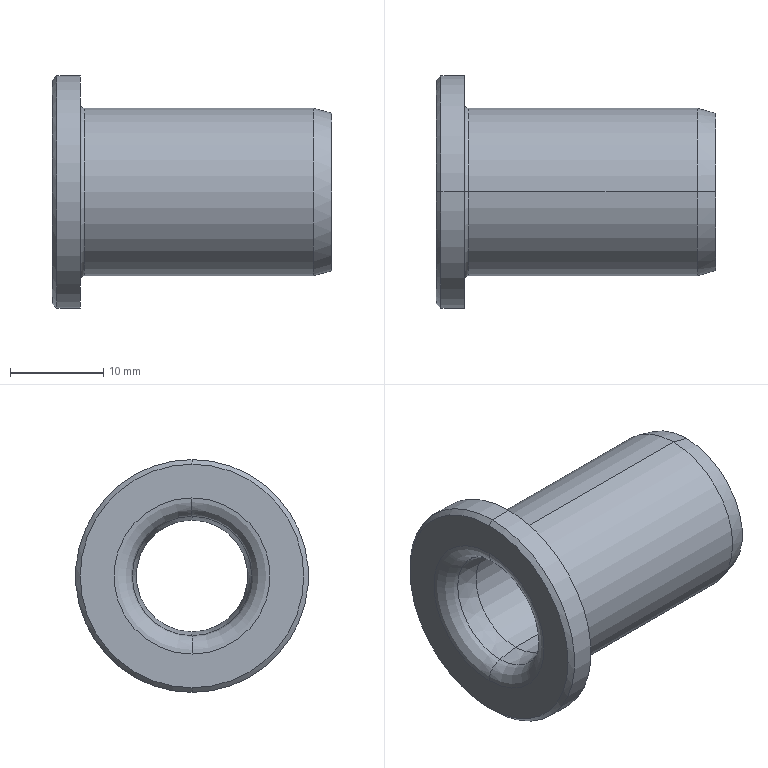Part | STEP file | 001-009-OFN01-d12-L30 | 1 solid | 23 faces | box 30 x 25 x 25 mm | volume 4819 mm3 | cone 8 | torus 6 | cylinder 6 | plane 3 | commonest cylinder face diameters 12 x2 18 x2 25 x2
STEP:
#1=CARTESIAN_POINT('',(0.,0.,0.));
#2=DIRECTION('',(0.,0.,1.));
#3=DIRECTION('',(1.,0.,0.));
#4=AXIS2_PLACEMENT_3D('',#1,#2,#3);
#5=CARTESIAN_POINT('',(0.,0.,-12.));
#6=VERTEX_POINT('',#5);
#7=CARTESIAN_POINT('',(0.,0.,12.));
#8=VERTEX_POINT('',#7);
#9=CARTESIAN_POINT('',(0.,0.,0.));
#10=DIRECTION('',(1.,0.,0.));
#11=DIRECTION('',(0.,0.,-1.));
#12=AXIS2_PLACEMENT_3D('',#9,#10,#11);
#13=CIRCLE('',#12,12.);
#14=CARTESIAN_POINT('',(0.5,0.,0.));
#15=DIRECTION('',(1.,0.,0.));
#16=DIRECTION('',(0.,0.,-1.));
#17=AXIS2_PLACEMENT_3D('',#14,#15,#16);
#18=CONICAL_SURFACE('',#17,12.5,0.7854);
#19=CARTESIAN_POINT('',(0.,-0.5));
#20=DIRECTION('',(1.,0.));
#21=VECTOR('',#20,1.);
#22=LINE('',#19,#21);
#23=(GEOMETRIC_REPRESENTATION_CONTEXT(2)PARAMETRIC_REPRESENTATION_CONTEXT()REPRESENTATION_CONTEXT('',''));
#24=DEFINITIONAL_REPRESENTATION('',(#22),#23);
#25=PCURVE('',#18,#24);
#26=CARTESIAN_POINT('',(0.,12.,0.));
#27=DIRECTION('',(-1.,0.,0.));
#28=DIRECTION('',(0.,0.,1.));
#29=AXIS2_PLACEMENT_3D('',#26,#27,#28);
#30=PLANE('',#29);
#31=CARTESIAN_POINT('',(-12.,-12.));
#32=CARTESIAN_POINT('',(-12.,8.785));
#33=CARTESIAN_POINT('',(6.,-1.608));
#34=CARTESIAN_POINT('',(24.,-12.));
#35=CARTESIAN_POINT('',(6.,-22.392));
#36=CARTESIAN_POINT('',(-12.,-32.785));
#37=CARTESIAN_POINT('',(-12.,-12.));
#38=(BOUNDED_CURVE()B_SPLINE_CURVE(2,(#31,#32,#33,#34,#35,#36,#37),.UNSPECIFIED.,.T.,.F.)B_SPLINE_CURVE_WITH_KNOTS((1,2,2,2,2,1),(-2.094,0.,2.094,4.189,6.283,8.378),.UNSPECIFIED.)CURVE()GEOMETRIC_REPRESENTATION_ITEM()RATIONAL_B_SPLINE_CURVE((1.,0.5,1.,0.5,1.,0.5,1.))REPRESENTATION_ITEM(''));
#39=(GEOMETRIC_REPRESENTATION_CONTEXT(2)PARAMETRIC_REPRESENTATION_CONTEXT()REPRESENTATION_CONTEXT('',''));
#40=DEFINITIONAL_REPRESENTATION('',(#38),#39);
#41=PCURVE('',#30,#40);
#42=SURFACE_CURVE('',#13,(#25,#41),.PCURVE_S1.);
#43=EDGE_CURVE('',#6,#8,#42,.T.);
#44=ORIENTED_EDGE('',*,*,#43,.T.);
#45=CARTESIAN_POINT('',(0.5,0.,12.5));
#46=VERTEX_POINT('',#45);
#47=CARTESIAN_POINT('',(0.5,0.,12.5));
#48=DIRECTION('',(0.7071,0.,0.7071));
#49=VECTOR('',#48,1.);
#50=LINE('',#47,#49);
#51=CARTESIAN_POINT('',(3.142,0.));
#52=DIRECTION('',(0.,1.));
#53=VECTOR('',#52,1.);
#54=LINE('',#51,#53);
#55=(GEOMETRIC_REPRESENTATION_CONTEXT(2)PARAMETRIC_REPRESENTATION_CONTEXT()REPRESENTATION_CONTEXT('',''));
#56=DEFINITIONAL_REPRESENTATION('',(#54),#55);
#57=PCURVE('',#18,#56);
#58=CARTESIAN_POINT('',(0.5,0.,0.));
#59=DIRECTION('',(1.,0.,0.));
#60=DIRECTION('',(0.,0.,-1.));
#61=AXIS2_PLACEMENT_3D('',#58,#59,#60);
#62=CONICAL_SURFACE('',#61,12.5,0.7854);
#63=CARTESIAN_POINT('',(3.142,0.));
#64=DIRECTION('',(0.,1.));
#65=VECTOR('',#64,1.);
#66=LINE('',#63,#65);
#67=(GEOMETRIC_REPRESENTATION_CONTEXT(2)PARAMETRIC_REPRESENTATION_CONTEXT()REPRESENTATION_CONTEXT('',''));
#68=DEFINITIONAL_REPRESENTATION('',(#66),#67);
#69=PCURVE('',#62,#68);
#70=SURFACE_CURVE('',#50,(#57,#69),.PCURVE_S1.);
#71=EDGE_CURVE('',#8,#46,#70,.T.);
#72=ORIENTED_EDGE('',*,*,#71,.T.);
#73=CARTESIAN_POINT('',(0.5,0.,-12.5));
#74=VERTEX_POINT('',#73);
#75=CARTESIAN_POINT('',(0.5,0.,0.));
#76=DIRECTION('',(1.,0.,0.));
#77=DIRECTION('',(0.,0.,-1.));
#78=AXIS2_PLACEMENT_3D('',#75,#76,#77);
#79=CIRCLE('',#78,12.5);
#80=CARTESIAN_POINT('',(0.,0.));
#81=DIRECTION('',(1.,0.));
#82=VECTOR('',#81,1.);
#83=LINE('',#80,#82);
#84=(GEOMETRIC_REPRESENTATION_CONTEXT(2)PARAMETRIC_REPRESENTATION_CONTEXT()REPRESENTATION_CONTEXT('',''));
#85=DEFINITIONAL_REPRESENTATION('',(#83),#84);
#86=PCURVE('',#18,#85);
#87=CARTESIAN_POINT('',(30.,0.,0.));
#88=DIRECTION('',(-1.,0.,0.));
#89=DIRECTION('',(0.,0.,-1.));
#90=AXIS2_PLACEMENT_3D('',#87,#88,#89);
#91=CYLINDRICAL_SURFACE('',#90,12.5);
#92=CARTESIAN_POINT('',(6.283,29.5));
#93=DIRECTION('',(-1.,0.));
#94=VECTOR('',#93,1.);
#95=LINE('',#92,#94);
#96=(GEOMETRIC_REPRESENTATION_CONTEXT(2)PARAMETRIC_REPRESENTATION_CONTEXT()REPRESENTATION_CONTEXT('',''));
#97=DEFINITIONAL_REPRESENTATION('',(#95),#96);
#98=PCURVE('',#91,#97);
#99=SURFACE_CURVE('',#79,(#86,#98),.PCURVE_S1.);
#100=EDGE_CURVE('',#74,#46,#99,.T.);
#101=ORIENTED_EDGE('',*,*,#100,.F.);
#102=CARTESIAN_POINT('',(0.5,0.,-12.5));
#103=DIRECTION('',(0.7071,0.,-0.7071));
#104=VECTOR('',#103,1.);
#105=LINE('',#102,#104);
#106=CARTESIAN_POINT('',(0.,0.));
#107=DIRECTION('',(0.,1.));
#108=VECTOR('',#107,1.);
#109=LINE('',#106,#108);
#110=(GEOMETRIC_REPRESENTATION_CONTEXT(2)PARAMETRIC_REPRESENTATION_CONTEXT()REPRESENTATION_CONTEXT('',''));
#111=DEFINITIONAL_REPRESENTATION('',(#109),#110);
#112=PCURVE('',#18,#111);
#113=CARTESIAN_POINT('',(6.283,0.));
#114=DIRECTION('',(0.,1.));
#115=VECTOR('',#114,1.);
#116=LINE('',#113,#115);
#117=(GEOMETRIC_REPRESENTATION_CONTEXT(2)PARAMETRIC_REPRESENTATION_CONTEXT()REPRESENTATION_CONTEXT('',''));
#118=DEFINITIONAL_REPRESENTATION('',(#116),#117);
#119=PCURVE('',#62,#118);
#120=SURFACE_CURVE('',#105,(#112,#119),.PCURVE_S1.);
#121=EDGE_CURVE('',#6,#74,#120,.T.);
#122=ORIENTED_EDGE('',*,*,#121,.F.);
#123=EDGE_LOOP('',(#44,#72,#101,#122));
#124=FACE_BOUND('',#123,.T.);
#125=ADVANCED_FACE('',(#124),#18,.T.);
#126=CARTESIAN_POINT('',(1.653,0.,-6.414));
#127=VERTEX_POINT('',#126);
#128=CARTESIAN_POINT('',(1.653,0.,6.414));
#129=VERTEX_POINT('',#128);
#130=CARTESIAN_POINT('',(1.653,0.,0.));
#131=DIRECTION('',(1.,0.,0.));
#132=DIRECTION('',(0.,0.,-1.));
#133=AXIS2_PLACEMENT_3D('',#130,#131,#132);
#134=CIRCLE('',#133,6.414);
#135=CARTESIAN_POINT('',(2.,0.,0.));
#136=DIRECTION('',(1.,0.,0.));
#137=DIRECTION('',(0.,0.,-1.));
#138=AXIS2_PLACEMENT_3D('',#135,#136,#137);
#139=TOROIDAL_SURFACE('',#138,8.384,2.);
#140=CARTESIAN_POINT('',(0.,3.316));
#141=DIRECTION('',(1.,0.));
#142=VECTOR('',#141,1.);
#143=LINE('',#140,#142);
#144=(GEOMETRIC_REPRESENTATION_CONTEXT(2)PARAMETRIC_REPRESENTATION_CONTEXT()REPRESENTATION_CONTEXT('',''));
#145=DEFINITIONAL_REPRESENTATION('',(#143),#144);
#146=PCURVE('',#139,#145);
#147=CARTESIAN_POINT('',(1.653,0.,0.));
#148=DIRECTION('',(-1.,0.,0.));
#149=DIRECTION('',(0.,0.,1.));
#150=AXIS2_PLACEMENT_3D('',#147,#148,#149);
#151=CONICAL_SURFACE('',#150,6.414,0.1745);
#152=CARTESIAN_POINT('',(3.142,0.));
#153=DIRECTION('',(-1.,0.));
#154=VECTOR('',#153,1.);
#155=LINE('',#152,#154);
#156=(GEOMETRIC_REPRESENTATION_CONTEXT(2)PARAMETRIC_REPRESENTATION_CONTEXT()REPRESENTATION_CONTEXT('',''));
#157=DEFINITIONAL_REPRESENTATION('',(#155),#156);
#158=PCURVE('',#151,#157);
#159=SURFACE_CURVE('',#134,(#146,#158),.PCURVE_S1.);
#160=EDGE_CURVE('',#127,#129,#159,.T.);
#161=ORIENTED_EDGE('',*,*,#160,.T.);
#162=CARTESIAN_POINT('',(0.,0.,8.384));
#163=VERTEX_POINT('',#162);
#164=CARTESIAN_POINT('',(2.,0.,8.384));
#165=DIRECTION('',(0.,1.,0.));
#166=DIRECTION('',(0.,0.,1.));
#167=AXIS2_PLACEMENT_3D('',#164,#165,#166);
#168=CIRCLE('',#167,2.);
#169=CARTESIAN_POINT('',(3.142,0.));
#170=DIRECTION('',(0.,1.));
#171=VECTOR('',#170,1.);
#172=LINE('',#169,#171);
#173=(GEOMETRIC_REPRESENTATION_CONTEXT(2)PARAMETRIC_REPRESENTATION_CONTEXT()REPRESENTATION_CONTEXT('',''));
#174=DEFINITIONAL_REPRESENTATION('',(#172),#173);
#175=PCURVE('',#139,#174);
#176=CARTESIAN_POINT('',(2.,0.,0.));
#177=DIRECTION('',(1.,0.,0.));
#178=DIRECTION('',(0.,0.,-1.));
#179=AXIS2_PLACEMENT_3D('',#176,#177,#178);
#180=TOROIDAL_SURFACE('',#179,8.384,2.);
#181=CARTESIAN_POINT('',(3.142,0.));
#182=DIRECTION('',(0.,1.));
#183=VECTOR('',#182,1.);
#184=LINE('',#181,#183);
#185=(GEOMETRIC_REPRESENTATION_CONTEXT(2)PARAMETRIC_REPRESENTATION_CONTEXT()REPRESENTATION_CONTEXT('',''));
#186=DEFINITIONAL_REPRESENTATION('',(#184),#185);
#187=PCURVE('',#180,#186);
#188=SURFACE_CURVE('',#168,(#175,#187),.PCURVE_S1.);
#189=EDGE_CURVE('',#129,#163,#188,.T.);
#190=ORIENTED_EDGE('',*,*,#189,.T.);
#191=CARTESIAN_POINT('',(0.,0.,-8.384));
#192=VERTEX_POINT('',#191);
#193=CARTESIAN_POINT('',(0.,0.,0.));
#194=DIRECTION('',(1.,0.,0.));
#195=DIRECTION('',(0.,0.,-1.));
#196=AXIS2_PLACEMENT_3D('',#193,#194,#195);
#197=CIRCLE('',#196,8.384);
#198=CARTESIAN_POINT('',(0.,4.712));
#199=DIRECTION('',(1.,0.));
#200=VECTOR('',#199,1.);
#201=LINE('',#198,#200);
#202=(GEOMETRIC_REPRESENTATION_CONTEXT(2)PARAMETRIC_REPRESENTATION_CONTEXT()REPRESENTATION_CONTEXT('',''));
#203=DEFINITIONAL_REPRESENTATION('',(#201),#202);
#204=PCURVE('',#139,#203);
#205=CARTESIAN_POINT('',(-8.384,-12.));
#206=CARTESIAN_POINT('',(-8.384,2.521));
#207=CARTESIAN_POINT('',(4.192,-4.74));
#208=CARTESIAN_POINT('',(16.767,-12.));
#209=CARTESIAN_POINT('',(4.192,-19.26));
#210=CARTESIAN_POINT('',(-8.384,-26.521));
#211=CARTESIAN_POINT('',(-8.384,-12.));
#212=(BOUNDED_CURVE()B_SPLINE_CURVE(2,(#205,#206,#207,#208,#209,#210,#211),.UNSPECIFIED.,.T.,.F.)B_SPLINE_CURVE_WITH_KNOTS((1,2,2,2,2,1),(-2.094,0.,2.094,4.189,6.283,8.378),.UNSPECIFIED.)CURVE()GEOMETRIC_REPRESENTATION_ITEM()RATIONAL_B_SPLINE_CURVE((1.,0.5,1.,0.5,1.,0.5,1.))REPRESENTATION_ITEM(''));
#213=(GEOMETRIC_REPRESENTATION_CONTEXT(2)PARAMETRIC_REPRESENTATION_CONTEXT()REPRESENTATION_CONTEXT('',''));
#214=DEFINITIONAL_REPRESENTATION('',(#212),#213);
#215=PCURVE('',#30,#214);
#216=SURFACE_CURVE('',#197,(#204,#215),.PCURVE_S1.);
#217=EDGE_CURVE('',#192,#163,#216,.T.);
#218=ORIENTED_EDGE('',*,*,#217,.F.);
#219=CARTESIAN_POINT('',(2.,0.,-8.384));
#220=DIRECTION('',(0.,-1.,0.));
#221=DIRECTION('',(0.,0.,-1.));
#222=AXIS2_PLACEMENT_3D('',#219,#220,#221);
#223=CIRCLE('',#222,2.);
#224=CARTESIAN_POINT('',(0.,0.));
#225=DIRECTION('',(0.,1.));
#226=VECTOR('',#225,1.);
#227=LINE('',#224,#226);
#228=(GEOMETRIC_REPRESENTATION_CONTEXT(2)PARAMETRIC_REPRESENTATION_CONTEXT()REPRESENTATION_CONTEXT('',''));
#229=DEFINITIONAL_REPRESENTATION('',(#227),#228);
#230=PCURVE('',#139,#229);
#231=CARTESIAN_POINT('',(6.283,0.));
#232=DIRECTION('',(0.,1.));
#233=VECTOR('',#232,1.);
#234=LINE('',#231,#233);
#235=(GEOMETRIC_REPRESENTATION_CONTEXT(2)PARAMETRIC_REPRESENTATION_CONTEXT()REPRESENTATION_CONTEXT('',''));
#236=DEFINITIONAL_REPRESENTATION('',(#234),#235);
#237=PCURVE('',#180,#236);
#238=SURFACE_CURVE('',#223,(#230,#237),.PCURVE_S1.);
#239=EDGE_CURVE('',#127,#192,#238,.T.);
#240=ORIENTED_EDGE('',*,*,#239,.F.);
#241=EDGE_LOOP('',(#161,#190,#218,#240));
#242=FACE_BOUND('',#241,.T.);
#243=ADVANCED_FACE('',(#242),#139,.T.);
#244=CARTESIAN_POINT('',(4.,0.,6.));
#245=VERTEX_POINT('',#244);
#246=CARTESIAN_POINT('',(1.653,0.,6.414));
#247=DIRECTION('',(-0.9848,0.,0.1736));
#248=VECTOR('',#247,1.);
#249=LINE('',#246,#248);
#250=CARTESIAN_POINT('',(1.653,0.,0.));
#251=DIRECTION('',(-1.,0.,0.));
#252=DIRECTION('',(0.,0.,1.));
#253=AXIS2_PLACEMENT_3D('',#250,#251,#252);
#254=CONICAL_SURFACE('',#253,6.414,0.1745);
#255=CARTESIAN_POINT('',(6.283,0.));
#256=DIRECTION('',(0.,1.));
#257=VECTOR('',#256,1.);
#258=LINE('',#255,#257);
#259=(GEOMETRIC_REPRESENTATION_CONTEXT(2)PARAMETRIC_REPRESENTATION_CONTEXT()REPRESENTATION_CONTEXT('',''));
#260=DEFINITIONAL_REPRESENTATION('',(#258),#259);
#261=PCURVE('',#254,#260);
#262=CARTESIAN_POINT('',(0.,0.));
#263=DIRECTION('',(0.,1.));
#264=VECTOR('',#263,1.);
#265=LINE('',#262,#264);
#266=(GEOMETRIC_REPRESENTATION_CONTEXT(2)PARAMETRIC_REPRESENTATION_CONTEXT()REPRESENTATION_CONTEXT('',''));
#267=DEFINITIONAL_REPRESENTATION('',(#265),#266);
#268=PCURVE('',#151,#267);
#269=SURFACE_CURVE('',#249,(#261,#268),.PCURVE_S1.);
#270=EDGE_CURVE('',#245,#129,#269,.T.);
#271=ORIENTED_EDGE('',*,*,#270,.T.);
#272=CARTESIAN_POINT('',(1.653,0.,0.));
#273=DIRECTION('',(1.,0.,0.));
#274=DIRECTION('',(0.,0.,-1.));
#275=AXIS2_PLACEMENT_3D('',#272,#273,#274);
#276=CIRCLE('',#275,6.414);
#277=CARTESIAN_POINT('',(9.425,0.));
#278=DIRECTION('',(-1.,0.));
#279=VECTOR('',#278,1.);
#280=LINE('',#277,#279);
#281=(GEOMETRIC_REPRESENTATION_CONTEXT(2)PARAMETRIC_REPRESENTATION_CONTEXT()REPRESENTATION_CONTEXT('',''));
#282=DEFINITIONAL_REPRESENTATION('',(#280),#281);
#283=PCURVE('',#254,#282);
#284=CARTESIAN_POINT('',(0.,3.316));
#285=DIRECTION('',(1.,0.));
#286=VECTOR('',#285,1.);
#287=LINE('',#284,#286);
#288=(GEOMETRIC_REPRESENTATION_CONTEXT(2)PARAMETRIC_REPRESENTATION_CONTEXT()REPRESENTATION_CONTEXT('',''));
#289=DEFINITIONAL_REPRESENTATION('',(#287),#288);
#290=PCURVE('',#180,#289);
#291=SURFACE_CURVE('',#276,(#283,#290),.PCURVE_S1.);
#292=EDGE_CURVE('',#129,#127,#291,.T.);
#293=ORIENTED_EDGE('',*,*,#292,.T.);
#294=CARTESIAN_POINT('',(4.,0.,-6.));
#295=VERTEX_POINT('',#294);
#296=CARTESIAN_POINT('',(1.653,0.,-6.414));
#297=DIRECTION('',(-0.9848,0.,-0.1736));
#298=VECTOR('',#297,1.);
#299=LINE('',#296,#298);
#300=CARTESIAN_POINT('',(3.142,0.));
#301=DIRECTION('',(0.,1.));
#302=VECTOR('',#301,1.);
#303=LINE('',#300,#302);
#304=(GEOMETRIC_REPRESENTATION_CONTEXT(2)PARAMETRIC_REPRESENTATION_CONTEXT()REPRESENTATION_CONTEXT('',''));
#305=DEFINITIONAL_REPRESENTATION('',(#303),#304);
#306=PCURVE('',#254,#305);
#307=CARTESIAN_POINT('',(3.142,0.));
#308=DIRECTION('',(0.,1.));
#309=VECTOR('',#308,1.);
#310=LINE('',#307,#309);
#311=(GEOMETRIC_REPRESENTATION_CONTEXT(2)PARAMETRIC_REPRESENTATION_CONTEXT()REPRESENTATION_CONTEXT('',''));
#312=DEFINITIONAL_REPRESENTATION('',(#310),#311);
#313=PCURVE('',#151,#312);
#314=SURFACE_CURVE('',#299,(#306,#313),.PCURVE_S1.);
#315=EDGE_CURVE('',#295,#127,#314,.T.);
#316=ORIENTED_EDGE('',*,*,#315,.F.);
#317=CARTESIAN_POINT('',(4.,0.,0.));
#318=DIRECTION('',(1.,0.,0.));
#319=DIRECTION('',(0.,0.,-1.));
#320=AXIS2_PLACEMENT_3D('',#317,#318,#319);
#321=CIRCLE('',#320,6.);
#322=CARTESIAN_POINT('',(9.425,-2.347));
#323=DIRECTION('',(-1.,0.));
#324=VECTOR('',#323,1.);
#325=LINE('',#322,#324);
#326=(GEOMETRIC_REPRESENTATION_CONTEXT(2)PARAMETRIC_REPRESENTATION_CONTEXT()REPRESENTATION_CONTEXT('',''));
#327=DEFINITIONAL_REPRESENTATION('',(#325),#326);
#328=PCURVE('',#254,#327);
#329=CARTESIAN_POINT('',(30.,0.,0.));
#330=DIRECTION('',(-1.,0.,0.));
#331=DIRECTION('',(0.,0.,-1.));
#332=AXIS2_PLACEMENT_3D('',#329,#330,#331);
#333=CYLINDRICAL_SURFACE('',#332,6.);
#334=CARTESIAN_POINT('',(6.283,26.));
#335=DIRECTION('',(-1.,0.));
#336=VECTOR('',#335,1.);
#337=LINE('',#334,#336);
#338=(GEOMETRIC_REPRESENTATION_CONTEXT(2)PARAMETRIC_REPRESENTATION_CONTEXT()REPRESENTATION_CONTEXT('',''));
#339=DEFINITIONAL_REPRESENTATION('',(#337),#338);
#340=PCURVE('',#333,#339);
#341=SURFACE_CURVE('',#321,(#328,#340),.PCURVE_S1.);
#342=EDGE_CURVE('',#245,#295,#341,.T.);
#343=ORIENTED_EDGE('',*,*,#342,.F.);
#344=EDGE_LOOP('',(#271,#293,#316,#343));
#345=FACE_BOUND('',#344,.F.);
#346=ADVANCED_FACE('',(#345),#254,.F.);
#347=CARTESIAN_POINT('',(28.,0.,-6.));
#348=VERTEX_POINT('',#347);
#349=CARTESIAN_POINT('',(30.,0.,-6.));
#350=DIRECTION('',(-1.,0.,0.));
#351=VECTOR('',#350,1.);
#352=LINE('',#349,#351);
#353=CARTESIAN_POINT('',(30.,0.,0.));
#354=DIRECTION('',(-1.,0.,0.));
#355=DIRECTION('',(0.,0.,-1.));
#356=AXIS2_PLACEMENT_3D('',#353,#354,#355);
#357=CYLINDRICAL_SURFACE('',#356,6.);
#358=CARTESIAN_POINT('',(6.283,0.));
#359=DIRECTION('',(0.,1.));
#360=VECTOR('',#359,1.);
#361=LINE('',#358,#360);
#362=(GEOMETRIC_REPRESENTATION_CONTEXT(2)PARAMETRIC_REPRESENTATION_CONTEXT()REPRESENTATION_CONTEXT('',''));
#363=DEFINITIONAL_REPRESENTATION('',(#361),#362);
#364=PCURVE('',#357,#363);
#365=CARTESIAN_POINT('',(0.,0.));
#366=DIRECTION('',(0.,1.));
#367=VECTOR('',#366,1.);
#368=LINE('',#365,#367);
#369=(GEOMETRIC_REPRESENTATION_CONTEXT(2)PARAMETRIC_REPRESENTATION_CONTEXT()REPRESENTATION_CONTEXT('',''));
#370=DEFINITIONAL_REPRESENTATION('',(#368),#369);
#371=PCURVE('',#333,#370);
#372=SURFACE_CURVE('',#352,(#364,#371),.PCURVE_S1.);
#373=EDGE_CURVE('',#348,#295,#372,.T.);
#374=ORIENTED_EDGE('',*,*,#373,.T.);
#375=CARTESIAN_POINT('',(4.,0.,0.));
#376=DIRECTION('',(1.,0.,0.));
#377=DIRECTION('',(0.,0.,-1.));
#378=AXIS2_PLACEMENT_3D('',#375,#376,#377);
#379=CIRCLE('',#378,6.);
#380=CARTESIAN_POINT('',(6.283,26.));
#381=DIRECTION('',(-1.,0.));
#382=VECTOR('',#381,1.);
#383=LINE('',#380,#382);
#384=(GEOMETRIC_REPRESENTATION_CONTEXT(2)PARAMETRIC_REPRESENTATION_CONTEXT()REPRESENTATION_CONTEXT('',''));
#385=DEFINITIONAL_REPRESENTATION('',(#383),#384);
#386=PCURVE('',#357,#385);
#387=CARTESIAN_POINT('',(3.142,-2.347));
#388=DIRECTION('',(-1.,0.));
#389=VECTOR('',#388,1.);
#390=LINE('',#387,#389);
#391=(GEOMETRIC_REPRESENTATION_CONTEXT(2)PARAMETRIC_REPRESENTATION_CONTEXT()REPRESENTATION_CONTEXT('',''));
#392=DEFINITIONAL_REPRESENTATION('',(#390),#391);
#393=PCURVE('',#151,#392);
#394=SURFACE_CURVE('',#379,(#386,#393),.PCURVE_S1.);
#395=EDGE_CURVE('',#295,#245,#394,.T.);
#396=ORIENTED_EDGE('',*,*,#395,.T.);
#397=CARTESIAN_POINT('',(28.,0.,6.));
#398=VERTEX_POINT('',#397);
#399=CARTESIAN_POINT('',(30.,0.,6.));
#400=DIRECTION('',(-1.,0.,0.));
#401=VECTOR('',#400,1.);
#402=LINE('',#399,#401);
#403=CARTESIAN_POINT('',(3.142,0.));
#404=DIRECTION('',(0.,1.));
#405=VECTOR('',#404,1.);
#406=LINE('',#403,#405);
#407=(GEOMETRIC_REPRESENTATION_CONTEXT(2)PARAMETRIC_REPRESENTATION_CONTEXT()REPRESENTATION_CONTEXT('',''));
#408=DEFINITIONAL_REPRESENTATION('',(#406),#407);
#409=PCURVE('',#357,#408);
#410=CARTESIAN_POINT('',(3.142,0.));
#411=DIRECTION('',(0.,1.));
#412=VECTOR('',#411,1.);
#413=LINE('',#410,#412);
#414=(GEOMETRIC_REPRESENTATION_CONTEXT(2)PARAMETRIC_REPRESENTATION_CONTEXT()REPRESENTATION_CONTEXT('',''));
#415=DEFINITIONAL_REPRESENTATION('',(#413),#414);
#416=PCURVE('',#333,#415);
#417=SURFACE_CURVE('',#402,(#409,#416),.PCURVE_S1.);
#418=EDGE_CURVE('',#398,#245,#417,.T.);
#419=ORIENTED_EDGE('',*,*,#418,.F.);
#420=CARTESIAN_POINT('',(28.,0.,0.));
#421=DIRECTION('',(1.,0.,0.));
#422=DIRECTION('',(0.,0.,-1.));
#423=AXIS2_PLACEMENT_3D('',#420,#421,#422);
#424=CIRCLE('',#423,6.);
#425=CARTESIAN_POINT('',(6.283,2.));
#426=DIRECTION('',(-1.,0.));
#427=VECTOR('',#426,1.);
#428=LINE('',#425,#427);
#429=(GEOMETRIC_REPRESENTATION_CONTEXT(2)PARAMETRIC_REPRESENTATION_CONTEXT()REPRESENTATION_CONTEXT('',''));
#430=DEFINITIONAL_REPRESENTATION('',(#428),#429);
#431=PCURVE('',#357,#430);
#432=CARTESIAN_POINT('',(28.,0.,0.));
#433=DIRECTION('',(1.,0.,0.));
#434=DIRECTION('',(0.,0.,-1.));
#435=AXIS2_PLACEMENT_3D('',#432,#433,#434);
#436=CONICAL_SURFACE('',#435,6.,0.1745);
#437=CARTESIAN_POINT('',(0.,0.));
#438=DIRECTION('',(1.,0.));
#439=VECTOR('',#438,1.);
#440=LINE('',#437,#439);
#441=(GEOMETRIC_REPRESENTATION_CONTEXT(2)PARAMETRIC_REPRESENTATION_CONTEXT()REPRESENTATION_CONTEXT('',''));
#442=DEFINITIONAL_REPRESENTATION('',(#440),#441);
#443=PCURVE('',#436,#442);
#444=SURFACE_CURVE('',#424,(#431,#443),.PCURVE_S1.);
#445=EDGE_CURVE('',#348,#398,#444,.T.);
#446=ORIENTED_EDGE('',*,*,#445,.F.);
#447=EDGE_LOOP('',(#374,#396,#419,#446));
#448=FACE_BOUND('',#447,.F.);
#449=ADVANCED_FACE('',(#448),#357,.F.);
#450=CARTESIAN_POINT('',(29.587,0.,-6.28));
#451=VERTEX_POINT('',#450);
#452=CARTESIAN_POINT('',(28.,0.,-6.));
#453=DIRECTION('',(0.9848,0.,-0.1736));
#454=VECTOR('',#453,1.);
#455=LINE('',#452,#454);
#456=CARTESIAN_POINT('',(28.,0.,0.));
#457=DIRECTION('',(1.,0.,0.));
#458=DIRECTION('',(0.,0.,-1.));
#459=AXIS2_PLACEMENT_3D('',#456,#457,#458);
#460=CONICAL_SURFACE('',#459,6.,0.1745);
#461=CARTESIAN_POINT('',(6.283,0.));
#462=DIRECTION('',(0.,1.));
#463=VECTOR('',#462,1.);
#464=LINE('',#461,#463);
#465=(GEOMETRIC_REPRESENTATION_CONTEXT(2)PARAMETRIC_REPRESENTATION_CONTEXT()REPRESENTATION_CONTEXT('',''));
#466=DEFINITIONAL_REPRESENTATION('',(#464),#465);
#467=PCURVE('',#460,#466);
#468=CARTESIAN_POINT('',(0.,0.));
#469=DIRECTION('',(0.,1.));
#470=VECTOR('',#469,1.);
#471=LINE('',#468,#470);
#472=(GEOMETRIC_REPRESENTATION_CONTEXT(2)PARAMETRIC_REPRESENTATION_CONTEXT()REPRESENTATION_CONTEXT('',''));
#473=DEFINITIONAL_REPRESENTATION('',(#471),#472);
#474=PCURVE('',#436,#473);
#475=SURFACE_CURVE('',#455,(#467,#474),.PCURVE_S1.);
#476=EDGE_CURVE('',#348,#451,#475,.T.);
#477=ORIENTED_EDGE('',*,*,#476,.T.);
#478=CARTESIAN_POINT('',(29.587,0.,6.28));
#479=VERTEX_POINT('',#478);
#480=CARTESIAN_POINT('',(29.587,0.,0.));
#481=DIRECTION('',(1.,0.,0.));
#482=DIRECTION('',(0.,0.,-1.));
#483=AXIS2_PLACEMENT_3D('',#480,#481,#482);
#484=CIRCLE('',#483,6.28);
#485=CARTESIAN_POINT('',(0.,1.587));
#486=DIRECTION('',(1.,0.));
#487=VECTOR('',#486,1.);
#488=LINE('',#485,#487);
#489=(GEOMETRIC_REPRESENTATION_CONTEXT(2)PARAMETRIC_REPRESENTATION_CONTEXT()REPRESENTATION_CONTEXT('',''));
#490=DEFINITIONAL_REPRESENTATION('',(#488),#489);
#491=PCURVE('',#460,#490);
#492=CARTESIAN_POINT('',(29.5,0.,0.));
#493=DIRECTION('',(1.,0.,0.));
#494=DIRECTION('',(0.,0.,-1.));
#495=AXIS2_PLACEMENT_3D('',#492,#493,#494);
#496=TOROIDAL_SURFACE('',#495,6.772,0.5);
#497=CARTESIAN_POINT('',(0.,2.967));
#498=DIRECTION('',(1.,0.));
#499=VECTOR('',#498,1.);
#500=LINE('',#497,#499);
#501=(GEOMETRIC_REPRESENTATION_CONTEXT(2)PARAMETRIC_REPRESENTATION_CONTEXT()REPRESENTATION_CONTEXT('',''));
#502=DEFINITIONAL_REPRESENTATION('',(#500),#501);
#503=PCURVE('',#496,#502);
#504=SURFACE_CURVE('',#484,(#491,#503),.PCURVE_S1.);
#505=EDGE_CURVE('',#479,#451,#504,.T.);
#506=ORIENTED_EDGE('',*,*,#505,.F.);
#507=CARTESIAN_POINT('',(28.,0.,6.));
#508=DIRECTION('',(0.9848,0.,0.1736));
#509=VECTOR('',#508,1.);
#510=LINE('',#507,#509);
#511=CARTESIAN_POINT('',(3.142,0.));
#512=DIRECTION('',(0.,1.));
#513=VECTOR('',#512,1.);
#514=LINE('',#511,#513);
#515=(GEOMETRIC_REPRESENTATION_CONTEXT(2)PARAMETRIC_REPRESENTATION_CONTEXT()REPRESENTATION_CONTEXT('',''));
#516=DEFINITIONAL_REPRESENTATION('',(#514),#515);
#517=PCURVE('',#460,#516);
#518=CARTESIAN_POINT('',(3.142,0.));
#519=DIRECTION('',(0.,1.));
#520=VECTOR('',#519,1.);
#521=LINE('',#518,#520);
#522=(GEOMETRIC_REPRESENTATION_CONTEXT(2)PARAMETRIC_REPRESENTATION_CONTEXT()REPRESENTATION_CONTEXT('',''));
#523=DEFINITIONAL_REPRESENTATION('',(#521),#522);
#524=PCURVE('',#436,#523);
#525=SURFACE_CURVE('',#510,(#517,#524),.PCURVE_S1.);
#526=EDGE_CURVE('',#398,#479,#525,.T.);
#527=ORIENTED_EDGE('',*,*,#526,.F.);
#528=CARTESIAN_POINT('',(28.,0.,0.));
#529=DIRECTION('',(1.,0.,0.));
#530=DIRECTION('',(0.,0.,-1.));
#531=AXIS2_PLACEMENT_3D('',#528,#529,#530);
#532=CIRCLE('',#531,6.);
#533=CARTESIAN_POINT('',(0.,0.));
#534=DIRECTION('',(1.,0.));
#535=VECTOR('',#534,1.);
#536=LINE('',#533,#535);
#537=(GEOMETRIC_REPRESENTATION_CONTEXT(2)PARAMETRIC_REPRESENTATION_CONTEXT()REPRESENTATION_CONTEXT('',''));
#538=DEFINITIONAL_REPRESENTATION('',(#536),#537);
#539=PCURVE('',#460,#538);
#540=CARTESIAN_POINT('',(6.283,2.));
#541=DIRECTION('',(-1.,0.));
#542=VECTOR('',#541,1.);
#543=LINE('',#540,#542);
#544=(GEOMETRIC_REPRESENTATION_CONTEXT(2)PARAMETRIC_REPRESENTATION_CONTEXT()REPRESENTATION_CONTEXT('',''));
#545=DEFINITIONAL_REPRESENTATION('',(#543),#544);
#546=PCURVE('',#333,#545);
#547=SURFACE_CURVE('',#532,(#539,#546),.PCURVE_S1.);
#548=EDGE_CURVE('',#398,#348,#547,.T.);
#549=ORIENTED_EDGE('',*,*,#548,.T.);
#550=EDGE_LOOP('',(#477,#506,#527,#549));
#551=FACE_BOUND('',#550,.F.);
#552=ADVANCED_FACE('',(#551),#460,.F.);
#553=CARTESIAN_POINT('',(30.,0.,-6.772));
#554=VERTEX_POINT('',#553);
#555=CARTESIAN_POINT('',(30.,0.,6.772));
#556=VERTEX_POINT('',#555);
#557=CARTESIAN_POINT('',(30.,0.,0.));
#558=DIRECTION('',(1.,0.,0.));
#559=DIRECTION('',(0.,0.,-1.));
#560=AXIS2_PLACEMENT_3D('',#557,#558,#559);
#561=CIRCLE('',#560,6.772);
#562=CARTESIAN_POINT('',(29.5,0.,0.));
#563=DIRECTION('',(1.,0.,0.));
#564=DIRECTION('',(0.,0.,-1.));
#565=AXIS2_PLACEMENT_3D('',#562,#563,#564);
#566=TOROIDAL_SURFACE('',#565,6.772,0.5);
#567=CARTESIAN_POINT('',(0.,1.571));
#568=DIRECTION('',(1.,0.));
#569=VECTOR('',#568,1.);
#570=LINE('',#567,#569);
#571=(GEOMETRIC_REPRESENTATION_CONTEXT(2)PARAMETRIC_REPRESENTATION_CONTEXT()REPRESENTATION_CONTEXT('',''));
#572=DEFINITIONAL_REPRESENTATION('',(#570),#571);
#573=PCURVE('',#566,#572);
#574=CARTESIAN_POINT('',(30.,6.772,0.));
#575=DIRECTION('',(1.,0.,0.));
#576=DIRECTION('',(0.,1.,0.));
#577=AXIS2_PLACEMENT_3D('',#574,#575,#576);
#578=PLANE('',#577);
#579=CARTESIAN_POINT('',(-6.772,0.));
#580=DIRECTION('',(0.,-1.));
#581=AXIS2_PLACEMENT_2D('',#579,#580);
#582=CIRCLE('',#581,6.772);
#583=(GEOMETRIC_REPRESENTATION_CONTEXT(2)PARAMETRIC_REPRESENTATION_CONTEXT()REPRESENTATION_CONTEXT('',''));
#584=DEFINITIONAL_REPRESENTATION('',(#582),#583);
#585=PCURVE('',#578,#584);
#586=SURFACE_CURVE('',#561,(#573,#585),.PCURVE_S1.);
#587=EDGE_CURVE('',#554,#556,#586,.T.);
#588=ORIENTED_EDGE('',*,*,#587,.T.);
#589=CARTESIAN_POINT('',(29.5,0.,6.772));
#590=DIRECTION('',(0.,1.,0.));
#591=DIRECTION('',(0.,0.,1.));
#592=AXIS2_PLACEMENT_3D('',#589,#590,#591);
#593=CIRCLE('',#592,0.5);
#594=CARTESIAN_POINT('',(3.142,0.));
#595=DIRECTION('',(0.,1.));
#596=VECTOR('',#595,1.);
#597=LINE('',#594,#596);
#598=(GEOMETRIC_REPRESENTATION_CONTEXT(2)PARAMETRIC_REPRESENTATION_CONTEXT()REPRESENTATION_CONTEXT('',''));
#599=DEFINITIONAL_REPRESENTATION('',(#597),#598);
#600=PCURVE('',#566,#599);
#601=CARTESIAN_POINT('',(3.142,0.));
#602=DIRECTION('',(0.,1.));
#603=VECTOR('',#602,1.);
#604=LINE('',#601,#603);
#605=(GEOMETRIC_REPRESENTATION_CONTEXT(2)PARAMETRIC_REPRESENTATION_CONTEXT()REPRESENTATION_CONTEXT('',''));
#606=DEFINITIONAL_REPRESENTATION('',(#604),#605);
#607=PCURVE('',#496,#606);
#608=SURFACE_CURVE('',#593,(#600,#607),.PCURVE_S1.);
#609=EDGE_CURVE('',#556,#479,#608,.T.);
#610=ORIENTED_EDGE('',*,*,#609,.T.);
#611=CARTESIAN_POINT('',(29.587,0.,0.));
#612=DIRECTION('',(1.,0.,0.));
#613=DIRECTION('',(0.,0.,-1.));
#614=AXIS2_PLACEMENT_3D('',#611,#612,#613);
#615=CIRCLE('',#614,6.28);
#616=CARTESIAN_POINT('',(0.,2.967));
#617=DIRECTION('',(1.,0.));
#618=VECTOR('',#617,1.);
#619=LINE('',#616,#618);
#620=(GEOMETRIC_REPRESENTATION_CONTEXT(2)PARAMETRIC_REPRESENTATION_CONTEXT()REPRESENTATION_CONTEXT('',''));
#621=DEFINITIONAL_REPRESENTATION('',(#619),#620);
#622=PCURVE('',#566,#621);
#623=CARTESIAN_POINT('',(0.,1.587));
#624=DIRECTION('',(1.,0.));
#625=VECTOR('',#624,1.);
#626=LINE('',#623,#625);
#627=(GEOMETRIC_REPRESENTATION_CONTEXT(2)PARAMETRIC_REPRESENTATION_CONTEXT()REPRESENTATION_CONTEXT('',''));
#628=DEFINITIONAL_REPRESENTATION('',(#626),#627);
#629=PCURVE('',#436,#628);
#630=SURFACE_CURVE('',#615,(#622,#629),.PCURVE_S1.);
#631=EDGE_CURVE('',#451,#479,#630,.T.);
#632=ORIENTED_EDGE('',*,*,#631,.F.);
#633=CARTESIAN_POINT('',(29.5,0.,-6.772));
#634=DIRECTION('',(0.,-1.,0.));
#635=DIRECTION('',(0.,0.,-1.));
#636=AXIS2_PLACEMENT_3D('',#633,#634,#635);
#637=CIRCLE('',#636,0.5);
#638=CARTESIAN_POINT('',(0.,0.));
#639=DIRECTION('',(0.,1.));
#640=VECTOR('',#639,1.);
#641=LINE('',#638,#640);
#642=(GEOMETRIC_REPRESENTATION_CONTEXT(2)PARAMETRIC_REPRESENTATION_CONTEXT()REPRESENTATION_CONTEXT('',''));
#643=DEFINITIONAL_REPRESENTATION('',(#641),#642);
#644=PCURVE('',#566,#643);
#645=CARTESIAN_POINT('',(6.283,0.));
#646=DIRECTION('',(0.,1.));
#647=VECTOR('',#646,1.);
#648=LINE('',#645,#647);
#649=(GEOMETRIC_REPRESENTATION_CONTEXT(2)PARAMETRIC_REPRESENTATION_CONTEXT()REPRESENTATION_CONTEXT('',''));
#650=DEFINITIONAL_REPRESENTATION('',(#648),#649);
#651=PCURVE('',#496,#650);
#652=SURFACE_CURVE('',#637,(#644,#651),.PCURVE_S1.);
#653=EDGE_CURVE('',#554,#451,#652,.T.);
#654=ORIENTED_EDGE('',*,*,#653,.F.);
#655=EDGE_LOOP('',(#588,#610,#632,#654));
#656=FACE_BOUND('',#655,.T.);
#657=ADVANCED_FACE('',(#656),#566,.T.);
#658=CARTESIAN_POINT('',(30.,0.,-8.464));
#659=VERTEX_POINT('',#658);
#660=CARTESIAN_POINT('',(30.,0.,8.464));
#661=VERTEX_POINT('',#660);
#662=CARTESIAN_POINT('',(30.,0.,0.));
#663=DIRECTION('',(1.,0.,0.));
#664=DIRECTION('',(0.,0.,-1.));
#665=AXIS2_PLACEMENT_3D('',#662,#663,#664);
#666=CIRCLE('',#665,8.464);
#667=CARTESIAN_POINT('',(30.,0.,0.));
#668=DIRECTION('',(-1.,0.,0.));
#669=DIRECTION('',(0.,0.,1.));
#670=AXIS2_PLACEMENT_3D('',#667,#668,#669);
#671=CONICAL_SURFACE('',#670,8.464,0.2618);
#672=CARTESIAN_POINT('',(3.142,0.));
#673=DIRECTION('',(-1.,0.));
#674=VECTOR('',#673,1.);
#675=LINE('',#672,#674);
#676=(GEOMETRIC_REPRESENTATION_CONTEXT(2)PARAMETRIC_REPRESENTATION_CONTEXT()REPRESENTATION_CONTEXT('',''));
#677=DEFINITIONAL_REPRESENTATION('',(#675),#676);
#678=PCURVE('',#671,#677);
#679=CARTESIAN_POINT('',(-6.772,0.));
#680=DIRECTION('',(0.,-1.));
#681=AXIS2_PLACEMENT_2D('',#679,#680);
#682=CIRCLE('',#681,8.464);
#683=(GEOMETRIC_REPRESENTATION_CONTEXT(2)PARAMETRIC_REPRESENTATION_CONTEXT()REPRESENTATION_CONTEXT('',''));
#684=DEFINITIONAL_REPRESENTATION('',(#682),#683);
#685=PCURVE('',#578,#684);
#686=SURFACE_CURVE('',#666,(#678,#685),.PCURVE_S1.);
#687=EDGE_CURVE('',#659,#661,#686,.T.);
#688=ORIENTED_EDGE('',*,*,#687,.F.);
#689=CARTESIAN_POINT('',(28.,0.,-9.));
#690=VERTEX_POINT('',#689);
#691=CARTESIAN_POINT('',(30.,0.,-8.464));
#692=DIRECTION('',(-0.9659,0.,-0.2588));
#693=VECTOR('',#692,1.);
#694=LINE('',#691,#693);
#695=CARTESIAN_POINT('',(3.142,0.));
#696=DIRECTION('',(0.,1.));
#697=VECTOR('',#696,1.);
#698=LINE('',#695,#697);
#699=(GEOMETRIC_REPRESENTATION_CONTEXT(2)PARAMETRIC_REPRESENTATION_CONTEXT()REPRESENTATION_CONTEXT('',''));
#700=DEFINITIONAL_REPRESENTATION('',(#698),#699);
#701=PCURVE('',#671,#700);
#702=CARTESIAN_POINT('',(30.,0.,0.));
#703=DIRECTION('',(-1.,0.,0.));
#704=DIRECTION('',(0.,0.,1.));
#705=AXIS2_PLACEMENT_3D('',#702,#703,#704);
#706=CONICAL_SURFACE('',#705,8.464,0.2618);
#707=CARTESIAN_POINT('',(3.142,0.));
#708=DIRECTION('',(0.,1.));
#709=VECTOR('',#708,1.);
#710=LINE('',#707,#709);
#711=(GEOMETRIC_REPRESENTATION_CONTEXT(2)PARAMETRIC_REPRESENTATION_CONTEXT()REPRESENTATION_CONTEXT('',''));
#712=DEFINITIONAL_REPRESENTATION('',(#710),#711);
#713=PCURVE('',#706,#712);
#714=SURFACE_CURVE('',#694,(#701,#713),.PCURVE_S1.);
#715=EDGE_CURVE('',#659,#690,#714,.T.);
#716=ORIENTED_EDGE('',*,*,#715,.T.);
#717=CARTESIAN_POINT('',(28.,0.,9.));
#718=VERTEX_POINT('',#717);
#719=CARTESIAN_POINT('',(28.,0.,0.));
#720=DIRECTION('',(1.,0.,0.));
#721=DIRECTION('',(0.,0.,-1.));
#722=AXIS2_PLACEMENT_3D('',#719,#720,#721);
#723=CIRCLE('',#722,9.);
#724=CARTESIAN_POINT('',(3.142,2.));
#725=DIRECTION('',(-1.,0.));
#726=VECTOR('',#725,1.);
#727=LINE('',#724,#726);
#728=(GEOMETRIC_REPRESENTATION_CONTEXT(2)PARAMETRIC_REPRESENTATION_CONTEXT()REPRESENTATION_CONTEXT('',''));
#729=DEFINITIONAL_REPRESENTATION('',(#727),#728);
#730=PCURVE('',#671,#729);
#731=CARTESIAN_POINT('',(30.,0.,0.));
#732=DIRECTION('',(-1.,0.,0.));
#733=DIRECTION('',(0.,0.,-1.));
#734=AXIS2_PLACEMENT_3D('',#731,#732,#733);
#735=CYLINDRICAL_SURFACE('',#734,9.);
#736=CARTESIAN_POINT('',(6.283,2.));
#737=DIRECTION('',(-1.,0.));
#738=VECTOR('',#737,1.);
#739=LINE('',#736,#738);
#740=(GEOMETRIC_REPRESENTATION_CONTEXT(2)PARAMETRIC_REPRESENTATION_CONTEXT()REPRESENTATION_CONTEXT('',''));
#741=DEFINITIONAL_REPRESENTATION('',(#739),#740);
#742=PCURVE('',#735,#741);
#743=SURFACE_CURVE('',#723,(#730,#742),.PCURVE_S1.);
#744=EDGE_CURVE('',#690,#718,#743,.T.);
#745=ORIENTED_EDGE('',*,*,#744,.T.);
#746=CARTESIAN_POINT('',(30.,0.,8.464));
#747=DIRECTION('',(-0.9659,0.,0.2588));
#748=VECTOR('',#747,1.);
#749=LINE('',#746,#748);
#750=CARTESIAN_POINT('',(0.,0.));
#751=DIRECTION('',(0.,1.));
#752=VECTOR('',#751,1.);
#753=LINE('',#750,#752);
#754=(GEOMETRIC_REPRESENTATION_CONTEXT(2)PARAMETRIC_REPRESENTATION_CONTEXT()REPRESENTATION_CONTEXT('',''));
#755=DEFINITIONAL_REPRESENTATION('',(#753),#754);
#756=PCURVE('',#671,#755);
#757=CARTESIAN_POINT('',(6.283,0.));
#758=DIRECTION('',(0.,1.));
#759=VECTOR('',#758,1.);
#760=LINE('',#757,#759);
#761=(GEOMETRIC_REPRESENTATION_CONTEXT(2)PARAMETRIC_REPRESENTATION_CONTEXT()REPRESENTATION_CONTEXT('',''));
#762=DEFINITIONAL_REPRESENTATION('',(#760),#761);
#763=PCURVE('',#706,#762);
#764=SURFACE_CURVE('',#749,(#756,#763),.PCURVE_S1.);
#765=EDGE_CURVE('',#661,#718,#764,.T.);
#766=ORIENTED_EDGE('',*,*,#765,.F.);
#767=EDGE_LOOP('',(#688,#716,#745,#766));
#768=FACE_BOUND('',#767,.T.);
#769=ADVANCED_FACE('',(#768),#671,.T.);
#770=CARTESIAN_POINT('',(28.,0.,0.));
#771=DIRECTION('',(1.,0.,0.));
#772=DIRECTION('',(0.,0.,-1.));
#773=AXIS2_PLACEMENT_3D('',#770,#771,#772);
#774=CIRCLE('',#773,9.);
#775=CARTESIAN_POINT('',(30.,0.,0.));
#776=DIRECTION('',(-1.,0.,0.));
#777=DIRECTION('',(0.,0.,-1.));
#778=AXIS2_PLACEMENT_3D('',#775,#776,#777);
#779=CYLINDRICAL_SURFACE('',#778,9.);
#780=CARTESIAN_POINT('',(6.283,2.));
#781=DIRECTION('',(-1.,0.));
#782=VECTOR('',#781,1.);
#783=LINE('',#780,#782);
#784=(GEOMETRIC_REPRESENTATION_CONTEXT(2)PARAMETRIC_REPRESENTATION_CONTEXT()REPRESENTATION_CONTEXT('',''));
#785=DEFINITIONAL_REPRESENTATION('',(#783),#784);
#786=PCURVE('',#779,#785);
#787=CARTESIAN_POINT('',(9.425,2.));
#788=DIRECTION('',(-1.,0.));
#789=VECTOR('',#788,1.);
#790=LINE('',#787,#789);
#791=(GEOMETRIC_REPRESENTATION_CONTEXT(2)PARAMETRIC_REPRESENTATION_CONTEXT()REPRESENTATION_CONTEXT('',''));
#792=DEFINITIONAL_REPRESENTATION('',(#790),#791);
#793=PCURVE('',#706,#792);
#794=SURFACE_CURVE('',#774,(#786,#793),.PCURVE_S1.);
#795=EDGE_CURVE('',#718,#690,#794,.T.);
#796=ORIENTED_EDGE('',*,*,#795,.F.);
#797=CARTESIAN_POINT('',(3.5,0.,9.));
#798=VERTEX_POINT('',#797);
#799=CARTESIAN_POINT('',(30.,0.,9.));
#800=DIRECTION('',(-1.,0.,0.));
#801=VECTOR('',#800,1.);
#802=LINE('',#799,#801);
#803=CARTESIAN_POINT('',(3.142,0.));
#804=DIRECTION('',(0.,1.));
#805=VECTOR('',#804,1.);
#806=LINE('',#803,#805);
#807=(GEOMETRIC_REPRESENTATION_CONTEXT(2)PARAMETRIC_REPRESENTATION_CONTEXT()REPRESENTATION_CONTEXT('',''));
#808=DEFINITIONAL_REPRESENTATION('',(#806),#807);
#809=PCURVE('',#779,#808);
#810=CARTESIAN_POINT('',(3.142,0.));
#811=DIRECTION('',(0.,1.));
#812=VECTOR('',#811,1.);
#813=LINE('',#810,#812);
#814=(GEOMETRIC_REPRESENTATION_CONTEXT(2)PARAMETRIC_REPRESENTATION_CONTEXT()REPRESENTATION_CONTEXT('',''));
#815=DEFINITIONAL_REPRESENTATION('',(#813),#814);
#816=PCURVE('',#735,#815);
#817=SURFACE_CURVE('',#802,(#809,#816),.PCURVE_S1.);
#818=EDGE_CURVE('',#718,#798,#817,.T.);
#819=ORIENTED_EDGE('',*,*,#818,.T.);
#820=CARTESIAN_POINT('',(3.5,0.,-9.));
#821=VERTEX_POINT('',#820);
#822=CARTESIAN_POINT('',(3.5,0.,0.));
#823=DIRECTION('',(1.,0.,0.));
#824=DIRECTION('',(0.,0.,-1.));
#825=AXIS2_PLACEMENT_3D('',#822,#823,#824);
#826=CIRCLE('',#825,9.);
#827=CARTESIAN_POINT('',(6.283,26.5));
#828=DIRECTION('',(-1.,0.));
#829=VECTOR('',#828,1.);
#830=LINE('',#827,#829);
#831=(GEOMETRIC_REPRESENTATION_CONTEXT(2)PARAMETRIC_REPRESENTATION_CONTEXT()REPRESENTATION_CONTEXT('',''));
#832=DEFINITIONAL_REPRESENTATION('',(#830),#831);
#833=PCURVE('',#779,#832);
#834=CARTESIAN_POINT('',(3.5,0.,0.));
#835=DIRECTION('',(1.,0.,0.));
#836=DIRECTION('',(0.,0.,-1.));
#837=AXIS2_PLACEMENT_3D('',#834,#835,#836);
#838=TOROIDAL_SURFACE('',#837,9.5,0.5);
#839=CARTESIAN_POINT('',(0.,3.142));
#840=DIRECTION('',(1.,0.));
#841=VECTOR('',#840,1.);
#842=LINE('',#839,#841);
#843=(GEOMETRIC_REPRESENTATION_CONTEXT(2)PARAMETRIC_REPRESENTATION_CONTEXT()REPRESENTATION_CONTEXT('',''));
#844=DEFINITIONAL_REPRESENTATION('',(#842),#843);
#845=PCURVE('',#838,#844);
#846=SURFACE_CURVE('',#826,(#833,#845),.PCURVE_S1.);
#847=EDGE_CURVE('',#798,#821,#846,.T.);
#848=ORIENTED_EDGE('',*,*,#847,.T.);
#849=CARTESIAN_POINT('',(30.,0.,-9.));
#850=DIRECTION('',(-1.,0.,0.));
#851=VECTOR('',#850,1.);
#852=LINE('',#849,#851);
#853=CARTESIAN_POINT('',(0.,0.));
#854=DIRECTION('',(0.,1.));
#855=VECTOR('',#854,1.);
#856=LINE('',#853,#855);
#857=(GEOMETRIC_REPRESENTATION_CONTEXT(2)PARAMETRIC_REPRESENTATION_CONTEXT()REPRESENTATION_CONTEXT('',''));
#858=DEFINITIONAL_REPRESENTATION('',(#856),#857);
#859=PCURVE('',#779,#858);
#860=CARTESIAN_POINT('',(6.283,0.));
#861=DIRECTION('',(0.,1.));
#862=VECTOR('',#861,1.);
#863=LINE('',#860,#862);
#864=(GEOMETRIC_REPRESENTATION_CONTEXT(2)PARAMETRIC_REPRESENTATION_CONTEXT()REPRESENTATION_CONTEXT('',''));
#865=DEFINITIONAL_REPRESENTATION('',(#863),#864);
#866=PCURVE('',#735,#865);
#867=SURFACE_CURVE('',#852,(#859,#866),.PCURVE_S1.);
#868=EDGE_CURVE('',#690,#821,#867,.T.);
#869=ORIENTED_EDGE('',*,*,#868,.F.);
#870=EDGE_LOOP('',(#796,#819,#848,#869));
#871=FACE_BOUND('',#870,.T.);
#872=ADVANCED_FACE('',(#871),#779,.T.);
#873=CARTESIAN_POINT('',(3.,0.,-9.5));
#874=VERTEX_POINT('',#873);
#875=CARTESIAN_POINT('',(3.5,0.,-9.5));
#876=DIRECTION('',(0.,-1.,0.));
#877=DIRECTION('',(0.,0.,-1.));
#878=AXIS2_PLACEMENT_3D('',#875,#876,#877);
#879=CIRCLE('',#878,0.5);
#880=CARTESIAN_POINT('',(6.283,0.));
#881=DIRECTION('',(0.,1.));
#882=VECTOR('',#881,1.);
#883=LINE('',#880,#882);
#884=(GEOMETRIC_REPRESENTATION_CONTEXT(2)PARAMETRIC_REPRESENTATION_CONTEXT()REPRESENTATION_CONTEXT('',''));
#885=DEFINITIONAL_REPRESENTATION('',(#883),#884);
#886=PCURVE('',#838,#885);
#887=CARTESIAN_POINT('',(3.5,0.,0.));
#888=DIRECTION('',(1.,0.,0.));
#889=DIRECTION('',(0.,0.,-1.));
#890=AXIS2_PLACEMENT_3D('',#887,#888,#889);
#891=TOROIDAL_SURFACE('',#890,9.5,0.5);
#892=CARTESIAN_POINT('',(0.,0.));
#893=DIRECTION('',(0.,1.));
#894=VECTOR('',#893,1.);
#895=LINE('',#892,#894);
#896=(GEOMETRIC_REPRESENTATION_CONTEXT(2)PARAMETRIC_REPRESENTATION_CONTEXT()REPRESENTATION_CONTEXT('',''));
#897=DEFINITIONAL_REPRESENTATION('',(#895),#896);
#898=PCURVE('',#891,#897);
#899=SURFACE_CURVE('',#879,(#886,#898),.PCURVE_S1.);
#900=EDGE_CURVE('',#821,#874,#899,.T.);
#901=ORIENTED_EDGE('',*,*,#900,.T.);
#902=CARTESIAN_POINT('',(3.,0.,9.5));
#903=VERTEX_POINT('',#902);
#904=CARTESIAN_POINT('',(3.,0.,0.));
#905=DIRECTION('',(1.,0.,0.));
#906=DIRECTION('',(0.,0.,-1.));
#907=AXIS2_PLACEMENT_3D('',#904,#905,#906);
#908=CIRCLE('',#907,9.5);
#909=CARTESIAN_POINT('',(0.,4.712));
#910=DIRECTION('',(1.,0.));
#911=VECTOR('',#910,1.);
#912=LINE('',#909,#911);
#913=(GEOMETRIC_REPRESENTATION_CONTEXT(2)PARAMETRIC_REPRESENTATION_CONTEXT()REPRESENTATION_CONTEXT('',''));
#914=DEFINITIONAL_REPRESENTATION('',(#912),#913);
#915=PCURVE('',#838,#914);
#916=CARTESIAN_POINT('',(3.,9.5,0.));
#917=DIRECTION('',(1.,0.,0.));
#918=DIRECTION('',(0.,1.,0.));
#919=AXIS2_PLACEMENT_3D('',#916,#917,#918);
#920=PLANE('',#919);
#921=CARTESIAN_POINT('',(-9.5,0.));
#922=DIRECTION('',(0.,-1.));
#923=AXIS2_PLACEMENT_2D('',#921,#922);
#924=CIRCLE('',#923,9.5);
#925=(GEOMETRIC_REPRESENTATION_CONTEXT(2)PARAMETRIC_REPRESENTATION_CONTEXT()REPRESENTATION_CONTEXT('',''));
#926=DEFINITIONAL_REPRESENTATION('',(#924),#925);
#927=PCURVE('',#920,#926);
#928=SURFACE_CURVE('',#908,(#915,#927),.PCURVE_S1.);
#929=EDGE_CURVE('',#903,#874,#928,.T.);
#930=ORIENTED_EDGE('',*,*,#929,.F.);
#931=CARTESIAN_POINT('',(3.5,0.,9.5));
#932=DIRECTION('',(0.,1.,0.));
#933=DIRECTION('',(0.,0.,1.));
#934=AXIS2_PLACEMENT_3D('',#931,#932,#933);
#935=CIRCLE('',#934,0.5);
#936=CARTESIAN_POINT('',(3.142,0.));
#937=DIRECTION('',(0.,1.));
#938=VECTOR('',#937,1.);
#939=LINE('',#936,#938);
#940=(GEOMETRIC_REPRESENTATION_CONTEXT(2)PARAMETRIC_REPRESENTATION_CONTEXT()REPRESENTATION_CONTEXT('',''));
#941=DEFINITIONAL_REPRESENTATION('',(#939),#940);
#942=PCURVE('',#838,#941);
#943=CARTESIAN_POINT('',(3.142,0.));
#944=DIRECTION('',(0.,1.));
#945=VECTOR('',#944,1.);
#946=LINE('',#943,#945);
#947=(GEOMETRIC_REPRESENTATION_CONTEXT(2)PARAMETRIC_REPRESENTATION_CONTEXT()REPRESENTATION_CONTEXT('',''));
#948=DEFINITIONAL_REPRESENTATION('',(#946),#947);
#949=PCURVE('',#891,#948);
#950=SURFACE_CURVE('',#935,(#942,#949),.PCURVE_S1.);
#951=EDGE_CURVE('',#798,#903,#950,.T.);
#952=ORIENTED_EDGE('',*,*,#951,.F.);
#953=ORIENTED_EDGE('',*,*,#847,.T.);
#954=EDGE_LOOP('',(#901,#930,#952,#953));
#955=FACE_BOUND('',#954,.F.);
#956=ADVANCED_FACE('',(#955),#838,.F.);
#957=CARTESIAN_POINT('',(3.,0.,12.5));
#958=VERTEX_POINT('',#957);
#959=CARTESIAN_POINT('',(3.,0.,-12.5));
#960=VERTEX_POINT('',#959);
#961=CARTESIAN_POINT('',(3.,0.,0.));
#962=DIRECTION('',(1.,0.,0.));
#963=DIRECTION('',(0.,0.,-1.));
#964=AXIS2_PLACEMENT_3D('',#961,#962,#963);
#965=CIRCLE('',#964,12.5);
#966=CARTESIAN_POINT('',(30.,0.,0.));
#967=DIRECTION('',(-1.,0.,0.));
#968=DIRECTION('',(0.,0.,-1.));
#969=AXIS2_PLACEMENT_3D('',#966,#967,#968);
#970=CYLINDRICAL_SURFACE('',#969,12.5);
#971=CARTESIAN_POINT('',(6.283,27.));
#972=DIRECTION('',(-1.,0.));
#973=VECTOR('',#972,1.);
#974=LINE('',#971,#973);
#975=(GEOMETRIC_REPRESENTATION_CONTEXT(2)PARAMETRIC_REPRESENTATION_CONTEXT()REPRESENTATION_CONTEXT('',''));
#976=DEFINITIONAL_REPRESENTATION('',(#974),#975);
#977=PCURVE('',#970,#976);
#978=CARTESIAN_POINT('',(-9.5,0.));
#979=DIRECTION('',(0.,-1.));
#980=AXIS2_PLACEMENT_2D('',#978,#979);
#981=CIRCLE('',#980,12.5);
#982=(GEOMETRIC_REPRESENTATION_CONTEXT(2)PARAMETRIC_REPRESENTATION_CONTEXT()REPRESENTATION_CONTEXT('',''));
#983=DEFINITIONAL_REPRESENTATION('',(#981),#982);
#984=PCURVE('',#920,#983);
#985=SURFACE_CURVE('',#965,(#977,#984),.PCURVE_S1.);
#986=EDGE_CURVE('',#958,#960,#985,.T.);
#987=ORIENTED_EDGE('',*,*,#986,.F.);
#988=CARTESIAN_POINT('',(30.,0.,12.5));
#989=DIRECTION('',(-1.,0.,0.));
#990=VECTOR('',#989,1.);
#991=LINE('',#988,#990);
#992=CARTESIAN_POINT('',(3.142,0.));
#993=DIRECTION('',(0.,1.));
#994=VECTOR('',#993,1.);
#995=LINE('',#992,#994);
#996=(GEOMETRIC_REPRESENTATION_CONTEXT(2)PARAMETRIC_REPRESENTATION_CONTEXT()REPRESENTATION_CONTEXT('',''));
#997=DEFINITIONAL_REPRESENTATION('',(#995),#996);
#998=PCURVE('',#970,#997);
#999=CARTESIAN_POINT('',(3.142,0.));
#1000=DIRECTION('',(0.,1.));
#1001=VECTOR('',#1000,1.);
#1002=LINE('',#999,#1001);
#1003=(GEOMETRIC_REPRESENTATION_CONTEXT(2)PARAMETRIC_REPRESENTATION_CONTEXT()REPRESENTATION_CONTEXT('',''));
#1004=DEFINITIONAL_REPRESENTATION('',(#1002),#1003);
#1005=PCURVE('',#91,#1004);
#1006=SURFACE_CURVE('',#991,(#998,#1005),.PCURVE_S1.);
#1007=EDGE_CURVE('',#958,#46,#1006,.T.);
#1008=ORIENTED_EDGE('',*,*,#1007,.T.);
#1009=CARTESIAN_POINT('',(0.5,0.,0.));
#1010=DIRECTION('',(1.,0.,0.));
#1011=DIRECTION('',(0.,0.,-1.));
#1012=AXIS2_PLACEMENT_3D('',#1009,#1010,#1011);
#1013=CIRCLE('',#1012,12.5);
#1014=CARTESIAN_POINT('',(6.283,29.5));
#1015=DIRECTION('',(-1.,0.));
#1016=VECTOR('',#1015,1.);
#1017=LINE('',#1014,#1016);
#1018=(GEOMETRIC_REPRESENTATION_CONTEXT(2)PARAMETRIC_REPRESENTATION_CONTEXT()REPRESENTATION_CONTEXT('',''));
#1019=DEFINITIONAL_REPRESENTATION('',(#1017),#1018);
#1020=PCURVE('',#970,#1019);
#1021=CARTESIAN_POINT('',(0.,0.));
#1022=DIRECTION('',(1.,0.));
#1023=VECTOR('',#1022,1.);
#1024=LINE('',#1021,#1023);
#1025=(GEOMETRIC_REPRESENTATION_CONTEXT(2)PARAMETRIC_REPRESENTATION_CONTEXT()REPRESENTATION_CONTEXT('',''));
#1026=DEFINITIONAL_REPRESENTATION('',(#1024),#1025);
#1027=PCURVE('',#62,#1026);
#1028=SURFACE_CURVE('',#1013,(#1020,#1027),.PCURVE_S1.);
#1029=EDGE_CURVE('',#46,#74,#1028,.T.);
#1030=ORIENTED_EDGE('',*,*,#1029,.T.);
#1031=CARTESIAN_POINT('',(30.,0.,-12.5));
#1032=DIRECTION('',(-1.,0.,0.));
#1033=VECTOR('',#1032,1.);
#1034=LINE('',#1031,#1033);
#1035=CARTESIAN_POINT('',(0.,0.));
#1036=DIRECTION('',(0.,1.));
#1037=VECTOR('',#1036,1.);
#1038=LINE('',#1035,#1037);
#1039=(GEOMETRIC_REPRESENTATION_CONTEXT(2)PARAMETRIC_REPRESENTATION_CONTEXT()REPRESENTATION_CONTEXT('',''));
#1040=DEFINITIONAL_REPRESENTATION('',(#1038),#1039);
#1041=PCURVE('',#970,#1040);
#1042=CARTESIAN_POINT('',(6.283,0.));
#1043=DIRECTION('',(0.,1.));
#1044=VECTOR('',#1043,1.);
#1045=LINE('',#1042,#1044);
#1046=(GEOMETRIC_REPRESENTATION_CONTEXT(2)PARAMETRIC_REPRESENTATION_CONTEXT()REPRESENTATION_CONTEXT('',''));
#1047=DEFINITIONAL_REPRESENTATION('',(#1045),#1046);
#1048=PCURVE('',#91,#1047);
#1049=SURFACE_CURVE('',#1034,(#1041,#1048),.PCURVE_S1.);
#1050=EDGE_CURVE('',#960,#74,#1049,.T.);
#1051=ORIENTED_EDGE('',*,*,#1050,.F.);
#1052=EDGE_LOOP('',(#987,#1008,#1030,#1051));
#1053=FACE_BOUND('',#1052,.T.);
#1054=ADVANCED_FACE('',(#1053),#970,.T.);
#1055=ORIENTED_EDGE('',*,*,#1007,.F.);
#1056=CARTESIAN_POINT('',(3.,0.,0.));
#1057=DIRECTION('',(1.,0.,0.));
#1058=DIRECTION('',(0.,0.,-1.));
#1059=AXIS2_PLACEMENT_3D('',#1056,#1057,#1058);
#1060=CIRCLE('',#1059,12.5);
#1061=CARTESIAN_POINT('',(6.283,27.));
#1062=DIRECTION('',(-1.,0.));
#1063=VECTOR('',#1062,1.);
#1064=LINE('',#1061,#1063);
#1065=(GEOMETRIC_REPRESENTATION_CONTEXT(2)PARAMETRIC_REPRESENTATION_CONTEXT()REPRESENTATION_CONTEXT('',''));
#1066=DEFINITIONAL_REPRESENTATION('',(#1064),#1065);
#1067=PCURVE('',#91,#1066);
#1068=CARTESIAN_POINT('',(-9.5,0.));
#1069=DIRECTION('',(0.,-1.));
#1070=AXIS2_PLACEMENT_2D('',#1068,#1069);
#1071=CIRCLE('',#1070,12.5);
#1072=(GEOMETRIC_REPRESENTATION_CONTEXT(2)PARAMETRIC_REPRESENTATION_CONTEXT()REPRESENTATION_CONTEXT('',''));
#1073=DEFINITIONAL_REPRESENTATION('',(#1071),#1072);
#1074=PCURVE('',#920,#1073);
#1075=SURFACE_CURVE('',#1060,(#1067,#1074),.PCURVE_S1.);
#1076=EDGE_CURVE('',#960,#958,#1075,.T.);
#1077=ORIENTED_EDGE('',*,*,#1076,.F.);
#1078=ORIENTED_EDGE('',*,*,#1050,.T.);
#1079=ORIENTED_EDGE('',*,*,#100,.T.);
#1080=EDGE_LOOP('',(#1055,#1077,#1078,#1079));
#1081=FACE_BOUND('',#1080,.T.);
#1082=ADVANCED_FACE('',(#1081),#91,.T.);
#1083=CARTESIAN_POINT('',(3.,0.,0.));
#1084=DIRECTION('',(1.,0.,0.));
#1085=DIRECTION('',(0.,0.,-1.));
#1086=AXIS2_PLACEMENT_3D('',#1083,#1084,#1085);
#1087=CIRCLE('',#1086,9.5);
#1088=CARTESIAN_POINT('',(-9.5,0.));
#1089=DIRECTION('',(0.,-1.));
#1090=AXIS2_PLACEMENT_2D('',#1088,#1089);
#1091=CIRCLE('',#1090,9.5);
#1092=(GEOMETRIC_REPRESENTATION_CONTEXT(2)PARAMETRIC_REPRESENTATION_CONTEXT()REPRESENTATION_CONTEXT('',''));
#1093=DEFINITIONAL_REPRESENTATION('',(#1091),#1092);
#1094=PCURVE('',#920,#1093);
#1095=CARTESIAN_POINT('',(0.,4.712));
#1096=DIRECTION('',(1.,0.));
#1097=VECTOR('',#1096,1.);
#1098=LINE('',#1095,#1097);
#1099=(GEOMETRIC_REPRESENTATION_CONTEXT(2)PARAMETRIC_REPRESENTATION_CONTEXT()REPRESENTATION_CONTEXT('',''));
#1100=DEFINITIONAL_REPRESENTATION('',(#1098),#1099);
#1101=PCURVE('',#891,#1100);
#1102=SURFACE_CURVE('',#1087,(#1094,#1101),.PCURVE_S1.);
#1103=EDGE_CURVE('',#874,#903,#1102,.T.);
#1104=ORIENTED_EDGE('',*,*,#1103,.F.);
#1105=ORIENTED_EDGE('',*,*,#929,.F.);
#1106=EDGE_LOOP('',(#1104,#1105));
#1107=FACE_BOUND('',#1106,.T.);
#1108=ORIENTED_EDGE('',*,*,#1076,.T.);
#1109=ORIENTED_EDGE('',*,*,#986,.T.);
#1110=EDGE_LOOP('',(#1108,#1109));
#1111=FACE_BOUND('',#1110,.T.);
#1112=ADVANCED_FACE('',(#1107,#1111),#920,.T.);
#1113=ORIENTED_EDGE('',*,*,#1103,.F.);
#1114=ORIENTED_EDGE('',*,*,#900,.F.);
#1115=CARTESIAN_POINT('',(3.5,0.,0.));
#1116=DIRECTION('',(1.,0.,0.));
#1117=DIRECTION('',(0.,0.,-1.));
#1118=AXIS2_PLACEMENT_3D('',#1115,#1116,#1117);
#1119=CIRCLE('',#1118,9.);
#1120=CARTESIAN_POINT('',(0.,3.142));
#1121=DIRECTION('',(1.,0.));
#1122=VECTOR('',#1121,1.);
#1123=LINE('',#1120,#1122);
#1124=(GEOMETRIC_REPRESENTATION_CONTEXT(2)PARAMETRIC_REPRESENTATION_CONTEXT()REPRESENTATION_CONTEXT('',''));
#1125=DEFINITIONAL_REPRESENTATION('',(#1123),#1124);
#1126=PCURVE('',#891,#1125);
#1127=CARTESIAN_POINT('',(6.283,26.5));
#1128=DIRECTION('',(-1.,0.));
#1129=VECTOR('',#1128,1.);
#1130=LINE('',#1127,#1129);
#1131=(GEOMETRIC_REPRESENTATION_CONTEXT(2)PARAMETRIC_REPRESENTATION_CONTEXT()REPRESENTATION_CONTEXT('',''));
#1132=DEFINITIONAL_REPRESENTATION('',(#1130),#1131);
#1133=PCURVE('',#735,#1132);
#1134=SURFACE_CURVE('',#1119,(#1126,#1133),.PCURVE_S1.);
#1135=EDGE_CURVE('',#821,#798,#1134,.T.);
#1136=ORIENTED_EDGE('',*,*,#1135,.T.);
#1137=ORIENTED_EDGE('',*,*,#951,.T.);
#1138=EDGE_LOOP('',(#1113,#1114,#1136,#1137));
#1139=FACE_BOUND('',#1138,.F.);
#1140=ADVANCED_FACE('',(#1139),#891,.F.);
#1141=ORIENTED_EDGE('',*,*,#818,.F.);
#1142=ORIENTED_EDGE('',*,*,#744,.F.);
#1143=ORIENTED_EDGE('',*,*,#868,.T.);
#1144=ORIENTED_EDGE('',*,*,#1135,.T.);
#1145=EDGE_LOOP('',(#1141,#1142,#1143,#1144));
#1146=FACE_BOUND('',#1145,.T.);
#1147=ADVANCED_FACE('',(#1146),#735,.T.);
#1148=ORIENTED_EDGE('',*,*,#715,.F.);
#1149=CARTESIAN_POINT('',(30.,0.,0.));
#1150=DIRECTION('',(1.,0.,0.));
#1151=DIRECTION('',(0.,0.,-1.));
#1152=AXIS2_PLACEMENT_3D('',#1149,#1150,#1151);
#1153=CIRCLE('',#1152,8.464);
#1154=CARTESIAN_POINT('',(9.425,0.));
#1155=DIRECTION('',(-1.,0.));
#1156=VECTOR('',#1155,1.);
#1157=LINE('',#1154,#1156);
#1158=(GEOMETRIC_REPRESENTATION_CONTEXT(2)PARAMETRIC_REPRESENTATION_CONTEXT()REPRESENTATION_CONTEXT('',''));
#1159=DEFINITIONAL_REPRESENTATION('',(#1157),#1158);
#1160=PCURVE('',#706,#1159);
#1161=CARTESIAN_POINT('',(-6.772,0.));
#1162=DIRECTION('',(0.,-1.));
#1163=AXIS2_PLACEMENT_2D('',#1161,#1162);
#1164=CIRCLE('',#1163,8.464);
#1165=(GEOMETRIC_REPRESENTATION_CONTEXT(2)PARAMETRIC_REPRESENTATION_CONTEXT()REPRESENTATION_CONTEXT('',''));
#1166=DEFINITIONAL_REPRESENTATION('',(#1164),#1165);
#1167=PCURVE('',#578,#1166);
#1168=SURFACE_CURVE('',#1153,(#1160,#1167),.PCURVE_S1.);
#1169=EDGE_CURVE('',#661,#659,#1168,.T.);
#1170=ORIENTED_EDGE('',*,*,#1169,.F.);
#1171=ORIENTED_EDGE('',*,*,#765,.T.);
#1172=ORIENTED_EDGE('',*,*,#795,.T.);
#1173=EDGE_LOOP('',(#1148,#1170,#1171,#1172));
#1174=FACE_BOUND('',#1173,.T.);
#1175=ADVANCED_FACE('',(#1174),#706,.T.);
#1176=ORIENTED_EDGE('',*,*,#587,.F.);
#1177=CARTESIAN_POINT('',(30.,0.,0.));
#1178=DIRECTION('',(1.,0.,0.));
#1179=DIRECTION('',(0.,0.,-1.));
#1180=AXIS2_PLACEMENT_3D('',#1177,#1178,#1179);
#1181=CIRCLE('',#1180,6.772);
#1182=CARTESIAN_POINT('',(-6.772,0.));
#1183=DIRECTION('',(0.,-1.));
#1184=AXIS2_PLACEMENT_2D('',#1182,#1183);
#1185=CIRCLE('',#1184,6.772);
#1186=(GEOMETRIC_REPRESENTATION_CONTEXT(2)PARAMETRIC_REPRESENTATION_CONTEXT()REPRESENTATION_CONTEXT('',''));
#1187=DEFINITIONAL_REPRESENTATION('',(#1185),#1186);
#1188=PCURVE('',#578,#1187);
#1189=CARTESIAN_POINT('',(0.,1.571));
#1190=DIRECTION('',(1.,0.));
#1191=VECTOR('',#1190,1.);
#1192=LINE('',#1189,#1191);
#1193=(GEOMETRIC_REPRESENTATION_CONTEXT(2)PARAMETRIC_REPRESENTATION_CONTEXT()REPRESENTATION_CONTEXT('',''));
#1194=DEFINITIONAL_REPRESENTATION('',(#1192),#1193);
#1195=PCURVE('',#496,#1194);
#1196=SURFACE_CURVE('',#1181,(#1188,#1195),.PCURVE_S1.);
#1197=EDGE_CURVE('',#556,#554,#1196,.T.);
#1198=ORIENTED_EDGE('',*,*,#1197,.F.);
#1199=EDGE_LOOP('',(#1176,#1198));
#1200=FACE_BOUND('',#1199,.T.);
#1201=ORIENTED_EDGE('',*,*,#1169,.T.);
#1202=ORIENTED_EDGE('',*,*,#687,.T.);
#1203=EDGE_LOOP('',(#1201,#1202));
#1204=FACE_BOUND('',#1203,.T.);
#1205=ADVANCED_FACE('',(#1200,#1204),#578,.T.);
#1206=ORIENTED_EDGE('',*,*,#609,.F.);
#1207=ORIENTED_EDGE('',*,*,#1197,.T.);
#1208=ORIENTED_EDGE('',*,*,#653,.T.);
#1209=ORIENTED_EDGE('',*,*,#505,.F.);
#1210=EDGE_LOOP('',(#1206,#1207,#1208,#1209));
#1211=FACE_BOUND('',#1210,.T.);
#1212=ADVANCED_FACE('',(#1211),#496,.T.);
#1213=ORIENTED_EDGE('',*,*,#631,.F.);
#1214=ORIENTED_EDGE('',*,*,#476,.F.);
#1215=ORIENTED_EDGE('',*,*,#445,.T.);
#1216=ORIENTED_EDGE('',*,*,#526,.T.);
#1217=EDGE_LOOP('',(#1213,#1214,#1215,#1216));
#1218=FACE_BOUND('',#1217,.F.);
#1219=ADVANCED_FACE('',(#1218),#436,.F.);
#1220=ORIENTED_EDGE('',*,*,#342,.T.);
#1221=ORIENTED_EDGE('',*,*,#373,.F.);
#1222=ORIENTED_EDGE('',*,*,#548,.F.);
#1223=ORIENTED_EDGE('',*,*,#418,.T.);
#1224=EDGE_LOOP('',(#1220,#1221,#1222,#1223));
#1225=FACE_BOUND('',#1224,.F.);
#1226=ADVANCED_FACE('',(#1225),#333,.F.);
#1227=ORIENTED_EDGE('',*,*,#160,.T.);
#1228=ORIENTED_EDGE('',*,*,#270,.F.);
#1229=ORIENTED_EDGE('',*,*,#395,.F.);
#1230=ORIENTED_EDGE('',*,*,#315,.T.);
#1231=EDGE_LOOP('',(#1227,#1228,#1229,#1230));
#1232=FACE_BOUND('',#1231,.F.);
#1233=ADVANCED_FACE('',(#1232),#151,.F.);
#1234=ORIENTED_EDGE('',*,*,#189,.F.);
#1235=ORIENTED_EDGE('',*,*,#292,.T.);
#1236=ORIENTED_EDGE('',*,*,#239,.T.);
#1237=CARTESIAN_POINT('',(0.,0.,0.));
#1238=DIRECTION('',(1.,0.,0.));
#1239=DIRECTION('',(0.,0.,-1.));
#1240=AXIS2_PLACEMENT_3D('',#1237,#1238,#1239);
#1241=CIRCLE('',#1240,8.384);
#1242=CARTESIAN_POINT('',(0.,4.712));
#1243=DIRECTION('',(1.,0.));
#1244=VECTOR('',#1243,1.);
#1245=LINE('',#1242,#1244);
#1246=(GEOMETRIC_REPRESENTATION_CONTEXT(2)PARAMETRIC_REPRESENTATION_CONTEXT()REPRESENTATION_CONTEXT('',''));
#1247=DEFINITIONAL_REPRESENTATION('',(#1245),#1246);
#1248=PCURVE('',#180,#1247);
#1249=CARTESIAN_POINT('',(-8.384,-12.));
#1250=CARTESIAN_POINT('',(-8.384,2.521));
#1251=CARTESIAN_POINT('',(4.192,-4.74));
#1252=CARTESIAN_POINT('',(16.767,-12.));
#1253=CARTESIAN_POINT('',(4.192,-19.26));
#1254=CARTESIAN_POINT('',(-8.384,-26.521));
#1255=CARTESIAN_POINT('',(-8.384,-12.));
#1256=(BOUNDED_CURVE()B_SPLINE_CURVE(2,(#1249,#1250,#1251,#1252,#1253,#1254,#1255),.UNSPECIFIED.,.T.,.F.)B_SPLINE_CURVE_WITH_KNOTS((1,2,2,2,2,1),(-2.094,0.,2.094,4.189,6.283,8.378),.UNSPECIFIED.)CURVE()GEOMETRIC_REPRESENTATION_ITEM()RATIONAL_B_SPLINE_CURVE((1.,0.5,1.,0.5,1.,0.5,1.))REPRESENTATION_ITEM(''));
#1257=(GEOMETRIC_REPRESENTATION_CONTEXT(2)PARAMETRIC_REPRESENTATION_CONTEXT()REPRESENTATION_CONTEXT('',''));
#1258=DEFINITIONAL_REPRESENTATION('',(#1256),#1257);
#1259=PCURVE('',#30,#1258);
#1260=SURFACE_CURVE('',#1241,(#1248,#1259),.PCURVE_S1.);
#1261=EDGE_CURVE('',#163,#192,#1260,.T.);
#1262=ORIENTED_EDGE('',*,*,#1261,.F.);
#1263=EDGE_LOOP('',(#1234,#1235,#1236,#1262));
#1264=FACE_BOUND('',#1263,.T.);
#1265=ADVANCED_FACE('',(#1264),#180,.T.);
#1266=ORIENTED_EDGE('',*,*,#217,.T.);
#1267=ORIENTED_EDGE('',*,*,#1261,.T.);
#1268=EDGE_LOOP('',(#1266,#1267));
#1269=FACE_BOUND('',#1268,.T.);
#1270=ORIENTED_EDGE('',*,*,#43,.F.);
#1271=CARTESIAN_POINT('',(0.,0.,0.));
#1272=DIRECTION('',(1.,0.,0.));
#1273=DIRECTION('',(0.,0.,-1.));
#1274=AXIS2_PLACEMENT_3D('',#1271,#1272,#1273);
#1275=CIRCLE('',#1274,12.);
#1276=CARTESIAN_POINT('',(-12.,-12.));
#1277=CARTESIAN_POINT('',(-12.,8.785));
#1278=CARTESIAN_POINT('',(6.,-1.608));
#1279=CARTESIAN_POINT('',(24.,-12.));
#1280=CARTESIAN_POINT('',(6.,-22.392));
#1281=CARTESIAN_POINT('',(-12.,-32.785));
#1282=CARTESIAN_POINT('',(-12.,-12.));
#1283=(BOUNDED_CURVE()B_SPLINE_CURVE(2,(#1276,#1277,#1278,#1279,#1280,#1281,#1282),.UNSPECIFIED.,.T.,.F.)B_SPLINE_CURVE_WITH_KNOTS((1,2,2,2,2,1),(-2.094,0.,2.094,4.189,6.283,8.378),.UNSPECIFIED.)CURVE()GEOMETRIC_REPRESENTATION_ITEM()RATIONAL_B_SPLINE_CURVE((1.,0.5,1.,0.5,1.,0.5,1.))REPRESENTATION_ITEM(''));
#1284=(GEOMETRIC_REPRESENTATION_CONTEXT(2)PARAMETRIC_REPRESENTATION_CONTEXT()REPRESENTATION_CONTEXT('',''));
#1285=DEFINITIONAL_REPRESENTATION('',(#1283),#1284);
#1286=PCURVE('',#30,#1285);
#1287=CARTESIAN_POINT('',(0.,-0.5));
#1288=DIRECTION('',(1.,0.));
#1289=VECTOR('',#1288,1.);
#1290=LINE('',#1287,#1289);
#1291=(GEOMETRIC_REPRESENTATION_CONTEXT(2)PARAMETRIC_REPRESENTATION_CONTEXT()REPRESENTATION_CONTEXT('',''));
#1292=DEFINITIONAL_REPRESENTATION('',(#1290),#1291);
#1293=PCURVE('',#62,#1292);
#1294=SURFACE_CURVE('',#1275,(#1286,#1293),.PCURVE_S1.);
#1295=EDGE_CURVE('',#8,#6,#1294,.T.);
#1296=ORIENTED_EDGE('',*,*,#1295,.F.);
#1297=EDGE_LOOP('',(#1270,#1296));
#1298=FACE_BOUND('',#1297,.T.);
#1299=ADVANCED_FACE('',(#1269,#1298),#30,.T.);
#1300=ORIENTED_EDGE('',*,*,#71,.F.);
#1301=ORIENTED_EDGE('',*,*,#1295,.T.);
#1302=ORIENTED_EDGE('',*,*,#121,.T.);
#1303=ORIENTED_EDGE('',*,*,#1029,.F.);
#1304=EDGE_LOOP('',(#1300,#1301,#1302,#1303));
#1305=FACE_BOUND('',#1304,.T.);
#1306=ADVANCED_FACE('',(#1305),#62,.T.);
#1307=CLOSED_SHELL('',(#125,#243,#346,#449,#552,#657,#769,#872,#956,#1054,#1082,#1112,#1140,#1147,#1175,#1205,#1212,#1219,#1226,#1233,#1265,#1299,#1306));
#1308=MANIFOLD_SOLID_BREP('',#1307);
#1309=(LENGTH_UNIT()NAMED_UNIT(*)SI_UNIT(.MILLI.,.METRE.));
#1310=UNCERTAINTY_MEASURE_WITH_UNIT(LENGTH_MEASURE(0.0000001),#1309,'','');
#1311=(NAMED_UNIT(*)PLANE_ANGLE_UNIT()SI_UNIT($,.RADIAN.));
#1312=(NAMED_UNIT(*)SI_UNIT($,.STERADIAN.)SOLID_ANGLE_UNIT());
#1313=(GEOMETRIC_REPRESENTATION_CONTEXT(3)GLOBAL_UNCERTAINTY_ASSIGNED_CONTEXT((#1310))GLOBAL_UNIT_ASSIGNED_CONTEXT((#1309,#1311,#1312))REPRESENTATION_CONTEXT('',''));
#1314=ADVANCED_BREP_SHAPE_REPRESENTATION('',(#4,#1308),#1313);